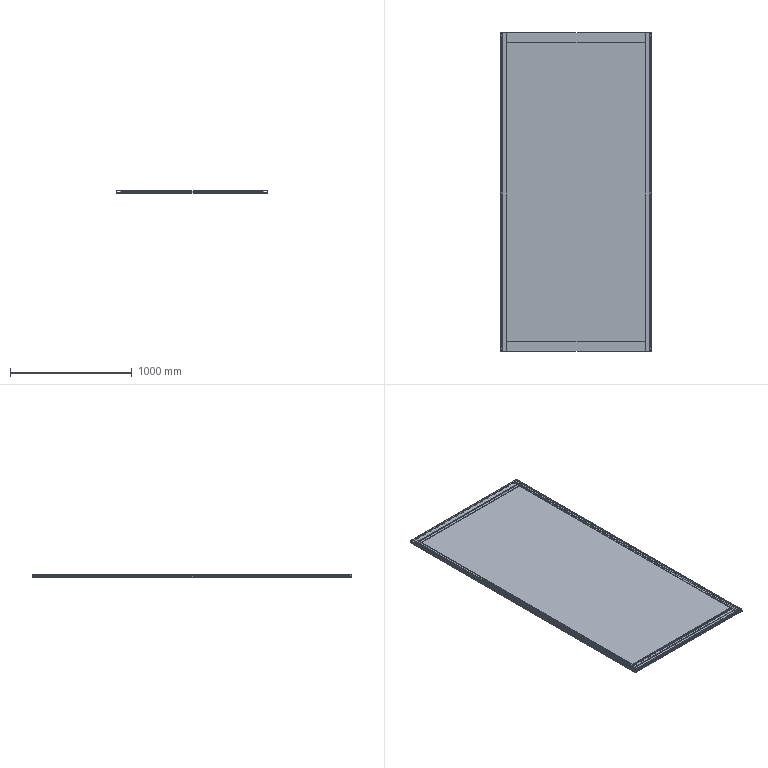Part | 5 solids | 465 faces | box 1240 x 2616 x 22 mm | volume 31291306 mm3 | plane 286 | cylinder 179 | commonest cylinder face diameters 1 x47 9 x40 0.4 x34 14 x20 7.2 x12 13 x12